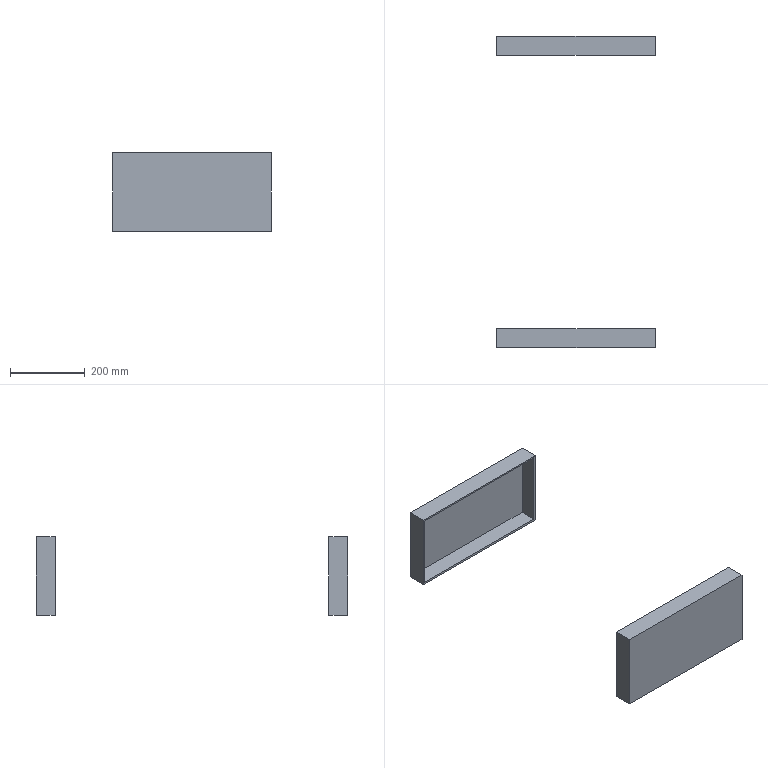Part | NX | features BREP 2 | 2 solids | 22 faces | box 422.751 x 830 x 210 mm | volume 1448252 mm3 | plane 22
STEP:
#1=CARTESIAN_POINT('',(-423.343,-172.553,205.));
#2=VERTEX_POINT('',#1);
#3=CARTESIAN_POINT('',(-423.343,-172.553,5.));
#4=VERTEX_POINT('',#3);
#5=CARTESIAN_POINT('',(-423.343,-172.553,210.));
#6=DIRECTION('',(0.,0.,-1.));
#7=VECTOR('',#6,1000.);
#8=LINE('',#5,#7);
#9=EDGE_CURVE('',#2,#4,#8,.T.);
#10=ORIENTED_EDGE('',*,*,#9,.F.);
#11=CARTESIAN_POINT('',(-423.343,-217.553,205.));
#12=VERTEX_POINT('',#11);
#13=CARTESIAN_POINT('',(-423.343,-167.553,205.));
#14=DIRECTION('',(0.,-1.,0.));
#15=VECTOR('',#14,1000.);
#16=LINE('',#13,#15);
#17=EDGE_CURVE('',#2,#12,#16,.T.);
#18=ORIENTED_EDGE('',*,*,#17,.T.);
#19=CARTESIAN_POINT('',(-423.343,-217.553,5.));
#20=VERTEX_POINT('',#19);
#21=CARTESIAN_POINT('',(-423.343,-217.553,210.));
#22=DIRECTION('',(0.,0.,1.));
#23=VECTOR('',#22,1000.);
#24=LINE('',#21,#23);
#25=EDGE_CURVE('',#20,#12,#24,.T.);
#26=ORIENTED_EDGE('',*,*,#25,.F.);
#27=CARTESIAN_POINT('',(-423.343,-167.553,5.));
#28=DIRECTION('',(0.,-1.,0.));
#29=VECTOR('',#28,1000.);
#30=LINE('',#27,#29);
#31=EDGE_CURVE('',#4,#20,#30,.T.);
#32=ORIENTED_EDGE('',*,*,#31,.F.);
#33=EDGE_LOOP('',(#10,#18,#26,#32));
#34=FACE_BOUND('',#33,.T.);
#35=CARTESIAN_POINT('',(-423.343,-167.553,210.));
#36=DIRECTION('',(1.,0.,0.));
#37=DIRECTION('',(0.,-1.,0.));
#38=AXIS2_PLACEMENT_3D('',#35,#36,#37);
#39=PLANE('',#38);
#40=ADVANCED_FACE('',(#34),#39,.T.);
#41=CARTESIAN_POINT('',(-10.592,-172.553,205.));
#42=VERTEX_POINT('',#41);
#43=CARTESIAN_POINT('',(-10.592,-172.553,5.));
#44=VERTEX_POINT('',#43);
#45=CARTESIAN_POINT('',(-10.592,-172.553,210.));
#46=DIRECTION('',(0.,0.,-1.));
#47=VECTOR('',#46,1000.);
#48=LINE('',#45,#47);
#49=EDGE_CURVE('',#42,#44,#48,.T.);
#50=ORIENTED_EDGE('',*,*,#49,.F.);
#51=CARTESIAN_POINT('',(-5.592,-172.553,205.));
#52=DIRECTION('',(-1.,0.,0.));
#53=VECTOR('',#52,1000.);
#54=LINE('',#51,#53);
#55=EDGE_CURVE('',#42,#2,#54,.T.);
#56=ORIENTED_EDGE('',*,*,#55,.T.);
#57=ORIENTED_EDGE('',*,*,#9,.T.);
#58=CARTESIAN_POINT('',(-5.592,-172.553,5.));
#59=DIRECTION('',(-1.,0.,0.));
#60=VECTOR('',#59,1000.);
#61=LINE('',#58,#60);
#62=EDGE_CURVE('',#44,#4,#61,.T.);
#63=ORIENTED_EDGE('',*,*,#62,.F.);
#64=EDGE_LOOP('',(#50,#56,#57,#63));
#65=FACE_BOUND('',#64,.T.);
#66=CARTESIAN_POINT('',(-5.592,-172.553,210.));
#67=DIRECTION('',(0.,-1.,0.));
#68=DIRECTION('',(-1.,0.,0.));
#69=AXIS2_PLACEMENT_3D('',#66,#67,#68);
#70=PLANE('',#69);
#71=ADVANCED_FACE('',(#65),#70,.T.);
#72=CARTESIAN_POINT('',(-10.592,-217.553,205.));
#73=VERTEX_POINT('',#72);
#74=CARTESIAN_POINT('',(-10.592,-217.553,5.));
#75=VERTEX_POINT('',#74);
#76=CARTESIAN_POINT('',(-10.592,-217.553,210.));
#77=DIRECTION('',(0.,0.,-1.));
#78=VECTOR('',#77,1000.);
#79=LINE('',#76,#78);
#80=EDGE_CURVE('',#73,#75,#79,.T.);
#81=ORIENTED_EDGE('',*,*,#80,.F.);
#82=CARTESIAN_POINT('',(-10.592,-217.553,205.));
#83=DIRECTION('',(0.,1.,0.));
#84=VECTOR('',#83,1000.);
#85=LINE('',#82,#84);
#86=EDGE_CURVE('',#73,#42,#85,.T.);
#87=ORIENTED_EDGE('',*,*,#86,.T.);
#88=ORIENTED_EDGE('',*,*,#49,.T.);
#89=CARTESIAN_POINT('',(-10.592,-217.553,5.));
#90=DIRECTION('',(0.,1.,0.));
#91=VECTOR('',#90,1000.);
#92=LINE('',#89,#91);
#93=EDGE_CURVE('',#75,#44,#92,.T.);
#94=ORIENTED_EDGE('',*,*,#93,.F.);
#95=EDGE_LOOP('',(#81,#87,#88,#94));
#96=FACE_BOUND('',#95,.T.);
#97=CARTESIAN_POINT('',(-10.592,-217.553,210.));
#98=DIRECTION('',(-1.,0.,0.));
#99=DIRECTION('',(0.,1.,0.));
#100=AXIS2_PLACEMENT_3D('',#97,#98,#99);
#101=PLANE('',#100);
#102=ADVANCED_FACE('',(#96),#101,.T.);
#103=CARTESIAN_POINT('',(-5.592,-217.553,210.));
#104=VERTEX_POINT('',#103);
#105=CARTESIAN_POINT('',(-428.343,-217.553,210.));
#106=VERTEX_POINT('',#105);
#107=CARTESIAN_POINT('',(-428.343,-217.553,210.));
#108=DIRECTION('',(-1.,0.,0.));
#109=VECTOR('',#108,1000.);
#110=LINE('',#107,#109);
#111=EDGE_CURVE('',#104,#106,#110,.T.);
#112=ORIENTED_EDGE('',*,*,#111,.F.);
#113=CARTESIAN_POINT('',(-5.592,-167.553,210.));
#114=VERTEX_POINT('',#113);
#115=CARTESIAN_POINT('',(-5.592,-217.553,210.));
#116=DIRECTION('',(0.,-1.,0.));
#117=VECTOR('',#116,1000.);
#118=LINE('',#115,#117);
#119=EDGE_CURVE('',#114,#104,#118,.T.);
#120=ORIENTED_EDGE('',*,*,#119,.F.);
#121=CARTESIAN_POINT('',(-428.343,-167.553,210.));
#122=VERTEX_POINT('',#121);
#123=CARTESIAN_POINT('',(-5.592,-167.553,210.));
#124=DIRECTION('',(1.,0.,0.));
#125=VECTOR('',#124,1000.);
#126=LINE('',#123,#125);
#127=EDGE_CURVE('',#122,#114,#126,.T.);
#128=ORIENTED_EDGE('',*,*,#127,.F.);
#129=CARTESIAN_POINT('',(-428.343,-167.553,210.));
#130=DIRECTION('',(0.,1.,0.));
#131=VECTOR('',#130,1000.);
#132=LINE('',#129,#131);
#133=EDGE_CURVE('',#106,#122,#132,.T.);
#134=ORIENTED_EDGE('',*,*,#133,.F.);
#135=EDGE_LOOP('',(#112,#120,#128,#134));
#136=FACE_BOUND('',#135,.T.);
#137=CARTESIAN_POINT('',(-428.343,-167.553,210.));
#138=DIRECTION('',(0.,0.,1.));
#139=DIRECTION('',(0.,1.,0.));
#140=AXIS2_PLACEMENT_3D('',#137,#138,#139);
#141=PLANE('',#140);
#142=ADVANCED_FACE('',(#136),#141,.T.);
#143=CARTESIAN_POINT('',(-5.592,-217.553,0.));
#144=VERTEX_POINT('',#143);
#145=CARTESIAN_POINT('',(-428.343,-217.553,0.));
#146=VERTEX_POINT('',#145);
#147=CARTESIAN_POINT('',(-428.343,-217.553,0.));
#148=DIRECTION('',(-1.,0.,0.));
#149=VECTOR('',#148,1000.);
#150=LINE('',#147,#149);
#151=EDGE_CURVE('',#144,#146,#150,.T.);
#152=ORIENTED_EDGE('',*,*,#151,.F.);
#153=CARTESIAN_POINT('',(-5.592,-217.553,210.));
#154=DIRECTION('',(0.,0.,-1.));
#155=VECTOR('',#154,1000.);
#156=LINE('',#153,#155);
#157=EDGE_CURVE('',#104,#144,#156,.T.);
#158=ORIENTED_EDGE('',*,*,#157,.F.);
#159=ORIENTED_EDGE('',*,*,#111,.T.);
#160=CARTESIAN_POINT('',(-428.343,-217.553,210.));
#161=DIRECTION('',(0.,0.,1.));
#162=VECTOR('',#161,1000.);
#163=LINE('',#160,#162);
#164=EDGE_CURVE('',#146,#106,#163,.T.);
#165=ORIENTED_EDGE('',*,*,#164,.F.);
#166=EDGE_LOOP('',(#152,#158,#159,#165));
#167=FACE_BOUND('',#166,.T.);
#168=ORIENTED_EDGE('',*,*,#80,.T.);
#169=CARTESIAN_POINT('',(-428.343,-217.553,5.));
#170=DIRECTION('',(1.,0.,0.));
#171=VECTOR('',#170,1000.);
#172=LINE('',#169,#171);
#173=EDGE_CURVE('',#20,#75,#172,.T.);
#174=ORIENTED_EDGE('',*,*,#173,.F.);
#175=ORIENTED_EDGE('',*,*,#25,.T.);
#176=CARTESIAN_POINT('',(-37.592,-217.553,205.));
#177=DIRECTION('',(1.,0.,0.));
#178=VECTOR('',#177,1000.);
#179=LINE('',#176,#178);
#180=EDGE_CURVE('',#12,#73,#179,.T.);
#181=ORIENTED_EDGE('',*,*,#180,.T.);
#182=EDGE_LOOP('',(#168,#174,#175,#181));
#183=FACE_BOUND('',#182,.T.);
#184=CARTESIAN_POINT('',(-428.343,-217.553,210.));
#185=DIRECTION('',(0.,-1.,0.));
#186=DIRECTION('',(0.,0.,1.));
#187=AXIS2_PLACEMENT_3D('',#184,#185,#186);
#188=PLANE('',#187);
#189=ADVANCED_FACE('',(#167,#183),#188,.T.);
#190=CARTESIAN_POINT('',(-5.592,-167.553,0.));
#191=VERTEX_POINT('',#190);
#192=CARTESIAN_POINT('',(-5.592,-217.553,0.));
#193=DIRECTION('',(0.,1.,0.));
#194=VECTOR('',#193,1000.);
#195=LINE('',#192,#194);
#196=EDGE_CURVE('',#144,#191,#195,.T.);
#197=ORIENTED_EDGE('',*,*,#196,.F.);
#198=ORIENTED_EDGE('',*,*,#151,.T.);
#199=CARTESIAN_POINT('',(-428.343,-167.553,0.));
#200=VERTEX_POINT('',#199);
#201=CARTESIAN_POINT('',(-428.343,-167.553,0.));
#202=DIRECTION('',(0.,-1.,0.));
#203=VECTOR('',#202,1000.);
#204=LINE('',#201,#203);
#205=EDGE_CURVE('',#200,#146,#204,.T.);
#206=ORIENTED_EDGE('',*,*,#205,.F.);
#207=CARTESIAN_POINT('',(-5.592,-167.553,0.));
#208=DIRECTION('',(-1.,0.,0.));
#209=VECTOR('',#208,1000.);
#210=LINE('',#207,#209);
#211=EDGE_CURVE('',#191,#200,#210,.T.);
#212=ORIENTED_EDGE('',*,*,#211,.F.);
#213=EDGE_LOOP('',(#197,#198,#206,#212));
#214=FACE_BOUND('',#213,.T.);
#215=CARTESIAN_POINT('',(-5.592,-167.553,0.));
#216=DIRECTION('',(0.,0.,1.));
#217=DIRECTION('',(1.,0.,0.));
#218=AXIS2_PLACEMENT_3D('',#215,#216,#217);
#219=PLANE('',#218);
#220=ADVANCED_FACE('',(#214),#219,.F.);
#221=CARTESIAN_POINT('',(-428.343,-167.553,210.));
#222=DIRECTION('',(0.,0.,-1.));
#223=VECTOR('',#222,1000.);
#224=LINE('',#221,#223);
#225=EDGE_CURVE('',#122,#200,#224,.T.);
#226=ORIENTED_EDGE('',*,*,#225,.T.);
#227=ORIENTED_EDGE('',*,*,#205,.T.);
#228=ORIENTED_EDGE('',*,*,#164,.T.);
#229=ORIENTED_EDGE('',*,*,#133,.T.);
#230=EDGE_LOOP('',(#226,#227,#228,#229));
#231=FACE_BOUND('',#230,.T.);
#232=CARTESIAN_POINT('',(-428.343,-167.553,210.));
#233=DIRECTION('',(1.,0.,0.));
#234=DIRECTION('',(0.,-1.,0.));
#235=AXIS2_PLACEMENT_3D('',#232,#233,#234);
#236=PLANE('',#235);
#237=ADVANCED_FACE('',(#231),#236,.F.);
#238=CARTESIAN_POINT('',(-5.592,-167.553,210.));
#239=DIRECTION('',(0.,0.,-1.));
#240=VECTOR('',#239,1000.);
#241=LINE('',#238,#240);
#242=EDGE_CURVE('',#114,#191,#241,.T.);
#243=ORIENTED_EDGE('',*,*,#242,.T.);
#244=ORIENTED_EDGE('',*,*,#211,.T.);
#245=ORIENTED_EDGE('',*,*,#225,.F.);
#246=ORIENTED_EDGE('',*,*,#127,.T.);
#247=EDGE_LOOP('',(#243,#244,#245,#246));
#248=FACE_BOUND('',#247,.T.);
#249=CARTESIAN_POINT('',(-5.592,-167.553,210.));
#250=DIRECTION('',(0.,-1.,0.));
#251=DIRECTION('',(-1.,0.,0.));
#252=AXIS2_PLACEMENT_3D('',#249,#250,#251);
#253=PLANE('',#252);
#254=ADVANCED_FACE('',(#248),#253,.F.);
#255=ORIENTED_EDGE('',*,*,#157,.T.);
#256=ORIENTED_EDGE('',*,*,#196,.T.);
#257=ORIENTED_EDGE('',*,*,#242,.F.);
#258=ORIENTED_EDGE('',*,*,#119,.T.);
#259=EDGE_LOOP('',(#255,#256,#257,#258));
#260=FACE_BOUND('',#259,.T.);
#261=CARTESIAN_POINT('',(-5.592,-217.553,210.));
#262=DIRECTION('',(-1.,0.,0.));
#263=DIRECTION('',(0.,1.,0.));
#264=AXIS2_PLACEMENT_3D('',#261,#262,#263);
#265=PLANE('',#264);
#266=ADVANCED_FACE('',(#260),#265,.F.);
#267=ORIENTED_EDGE('',*,*,#62,.T.);
#268=ORIENTED_EDGE('',*,*,#31,.T.);
#269=ORIENTED_EDGE('',*,*,#173,.T.);
#270=ORIENTED_EDGE('',*,*,#93,.T.);
#271=EDGE_LOOP('',(#267,#268,#269,#270));
#272=FACE_BOUND('',#271,.T.);
#273=CARTESIAN_POINT('',(0.,0.,5.));
#274=DIRECTION('',(0.,0.,1.));
#275=DIRECTION('',(-1.,0.,0.));
#276=AXIS2_PLACEMENT_3D('',#273,#274,#275);
#277=PLANE('',#276);
#278=ADVANCED_FACE('',(#272),#277,.T.);
#279=ORIENTED_EDGE('',*,*,#17,.F.);
#280=ORIENTED_EDGE('',*,*,#55,.F.);
#281=ORIENTED_EDGE('',*,*,#86,.F.);
#282=ORIENTED_EDGE('',*,*,#180,.F.);
#283=EDGE_LOOP('',(#279,#280,#281,#282));
#284=FACE_BOUND('',#283,.T.);
#285=CARTESIAN_POINT('',(0.,0.,205.));
#286=DIRECTION('',(0.,0.,1.));
#287=DIRECTION('',(-1.,0.,0.));
#288=AXIS2_PLACEMENT_3D('',#285,#286,#287);
#289=PLANE('',#288);
#290=ADVANCED_FACE('',(#284),#289,.F.);
#291=CLOSED_SHELL('',(#40,#71,#102,#142,#189,#220,#237,#254,#266,#278,#290));
#292=MANIFOLD_SOLID_BREP('',#291);
#293=CARTESIAN_POINT('',(-423.343,-992.553,205.));
#294=VERTEX_POINT('',#293);
#295=CARTESIAN_POINT('',(-423.343,-947.553,205.));
#296=VERTEX_POINT('',#295);
#297=CARTESIAN_POINT('',(-423.343,-997.553,205.));
#298=DIRECTION('',(0.,1.,0.));
#299=VECTOR('',#298,1000.);
#300=LINE('',#297,#299);
#301=EDGE_CURVE('',#294,#296,#300,.T.);
#302=ORIENTED_EDGE('',*,*,#301,.F.);
#303=CARTESIAN_POINT('',(-423.343,-992.553,5.));
#304=VERTEX_POINT('',#303);
#305=CARTESIAN_POINT('',(-423.343,-992.553,210.));
#306=DIRECTION('',(0.,0.,-1.));
#307=VECTOR('',#306,1000.);
#308=LINE('',#305,#307);
#309=EDGE_CURVE('',#294,#304,#308,.T.);
#310=ORIENTED_EDGE('',*,*,#309,.T.);
#311=CARTESIAN_POINT('',(-423.343,-947.553,5.));
#312=VERTEX_POINT('',#311);
#313=CARTESIAN_POINT('',(-423.343,-997.553,5.));
#314=DIRECTION('',(0.,-1.,0.));
#315=VECTOR('',#314,1000.);
#316=LINE('',#313,#315);
#317=EDGE_CURVE('',#312,#304,#316,.T.);
#318=ORIENTED_EDGE('',*,*,#317,.F.);
#319=CARTESIAN_POINT('',(-423.343,-947.553,210.));
#320=DIRECTION('',(0.,0.,1.));
#321=VECTOR('',#320,1000.);
#322=LINE('',#319,#321);
#323=EDGE_CURVE('',#312,#296,#322,.T.);
#324=ORIENTED_EDGE('',*,*,#323,.T.);
#325=EDGE_LOOP('',(#302,#310,#318,#324));
#326=FACE_BOUND('',#325,.T.);
#327=CARTESIAN_POINT('',(-423.343,-997.553,210.));
#328=DIRECTION('',(-1.,0.,0.));
#329=DIRECTION('',(0.,1.,0.));
#330=AXIS2_PLACEMENT_3D('',#327,#328,#329);
#331=PLANE('',#330);
#332=ADVANCED_FACE('',(#326),#331,.F.);
#333=CARTESIAN_POINT('',(-10.592,-992.553,205.));
#334=VERTEX_POINT('',#333);
#335=CARTESIAN_POINT('',(-5.592,-992.553,205.));
#336=DIRECTION('',(-1.,0.,0.));
#337=VECTOR('',#336,1000.);
#338=LINE('',#335,#337);
#339=EDGE_CURVE('',#334,#294,#338,.T.);
#340=ORIENTED_EDGE('',*,*,#339,.F.);
#341=CARTESIAN_POINT('',(-10.592,-992.553,5.));
#342=VERTEX_POINT('',#341);
#343=CARTESIAN_POINT('',(-10.592,-992.553,210.));
#344=DIRECTION('',(0.,0.,-1.));
#345=VECTOR('',#344,1000.);
#346=LINE('',#343,#345);
#347=EDGE_CURVE('',#334,#342,#346,.T.);
#348=ORIENTED_EDGE('',*,*,#347,.T.);
#349=CARTESIAN_POINT('',(-5.592,-992.553,5.));
#350=DIRECTION('',(1.,0.,0.));
#351=VECTOR('',#350,1000.);
#352=LINE('',#349,#351);
#353=EDGE_CURVE('',#304,#342,#352,.T.);
#354=ORIENTED_EDGE('',*,*,#353,.F.);
#355=ORIENTED_EDGE('',*,*,#309,.F.);
#356=EDGE_LOOP('',(#340,#348,#354,#355));
#357=FACE_BOUND('',#356,.T.);
#358=CARTESIAN_POINT('',(-5.592,-992.553,210.));
#359=DIRECTION('',(0.,-1.,0.));
#360=DIRECTION('',(-1.,0.,0.));
#361=AXIS2_PLACEMENT_3D('',#358,#359,#360);
#362=PLANE('',#361);
#363=ADVANCED_FACE('',(#357),#362,.F.);
#364=CARTESIAN_POINT('',(-10.592,-947.553,205.));
#365=VERTEX_POINT('',#364);
#366=CARTESIAN_POINT('',(-10.592,-947.553,205.));
#367=DIRECTION('',(0.,-1.,0.));
#368=VECTOR('',#367,1000.);
#369=LINE('',#366,#368);
#370=EDGE_CURVE('',#365,#334,#369,.T.);
#371=ORIENTED_EDGE('',*,*,#370,.F.);
#372=CARTESIAN_POINT('',(-10.592,-947.553,5.));
#373=VERTEX_POINT('',#372);
#374=CARTESIAN_POINT('',(-10.592,-947.553,210.));
#375=DIRECTION('',(0.,0.,-1.));
#376=VECTOR('',#375,1000.);
#377=LINE('',#374,#376);
#378=EDGE_CURVE('',#365,#373,#377,.T.);
#379=ORIENTED_EDGE('',*,*,#378,.T.);
#380=CARTESIAN_POINT('',(-10.592,-947.553,5.));
#381=DIRECTION('',(0.,1.,0.));
#382=VECTOR('',#381,1000.);
#383=LINE('',#380,#382);
#384=EDGE_CURVE('',#342,#373,#383,.T.);
#385=ORIENTED_EDGE('',*,*,#384,.F.);
#386=ORIENTED_EDGE('',*,*,#347,.F.);
#387=EDGE_LOOP('',(#371,#379,#385,#386));
#388=FACE_BOUND('',#387,.T.);
#389=CARTESIAN_POINT('',(-10.592,-947.553,210.));
#390=DIRECTION('',(1.,0.,0.));
#391=DIRECTION('',(0.,-1.,0.));
#392=AXIS2_PLACEMENT_3D('',#389,#390,#391);
#393=PLANE('',#392);
#394=ADVANCED_FACE('',(#388),#393,.F.);
#395=CARTESIAN_POINT('',(-428.343,-947.553,210.));
#396=VERTEX_POINT('',#395);
#397=CARTESIAN_POINT('',(-5.592,-947.553,210.));
#398=VERTEX_POINT('',#397);
#399=CARTESIAN_POINT('',(-5.592,-947.553,210.));
#400=DIRECTION('',(1.,0.,0.));
#401=VECTOR('',#400,1000.);
#402=LINE('',#399,#401);
#403=EDGE_CURVE('',#396,#398,#402,.T.);
#404=ORIENTED_EDGE('',*,*,#403,.F.);
#405=CARTESIAN_POINT('',(-428.343,-997.553,210.));
#406=VERTEX_POINT('',#405);
#407=CARTESIAN_POINT('',(-428.343,-997.553,210.));
#408=DIRECTION('',(0.,-1.,0.));
#409=VECTOR('',#408,1000.);
#410=LINE('',#407,#409);
#411=EDGE_CURVE('',#396,#406,#410,.T.);
#412=ORIENTED_EDGE('',*,*,#411,.T.);
#413=CARTESIAN_POINT('',(-5.592,-997.553,210.));
#414=VERTEX_POINT('',#413);
#415=CARTESIAN_POINT('',(-5.592,-997.553,210.));
#416=DIRECTION('',(1.,0.,0.));
#417=VECTOR('',#416,1000.);
#418=LINE('',#415,#417);
#419=EDGE_CURVE('',#406,#414,#418,.T.);
#420=ORIENTED_EDGE('',*,*,#419,.T.);
#421=CARTESIAN_POINT('',(-5.592,-947.553,210.));
#422=DIRECTION('',(0.,1.,0.));
#423=VECTOR('',#422,1000.);
#424=LINE('',#421,#423);
#425=EDGE_CURVE('',#414,#398,#424,.T.);
#426=ORIENTED_EDGE('',*,*,#425,.T.);
#427=EDGE_LOOP('',(#404,#412,#420,#426));
#428=FACE_BOUND('',#427,.T.);
#429=CARTESIAN_POINT('',(-5.592,-947.553,210.));
#430=DIRECTION('',(0.,0.,1.));
#431=DIRECTION('',(0.,1.,0.));
#432=AXIS2_PLACEMENT_3D('',#429,#430,#431);
#433=PLANE('',#432);
#434=ADVANCED_FACE('',(#428),#433,.T.);
#435=CARTESIAN_POINT('',(-428.343,-947.553,0.));
#436=VERTEX_POINT('',#435);
#437=CARTESIAN_POINT('',(-5.592,-947.553,0.));
#438=VERTEX_POINT('',#437);
#439=CARTESIAN_POINT('',(-428.343,-947.553,0.));
#440=DIRECTION('',(1.,0.,0.));
#441=VECTOR('',#440,1000.);
#442=LINE('',#439,#441);
#443=EDGE_CURVE('',#436,#438,#442,.T.);
#444=ORIENTED_EDGE('',*,*,#443,.T.);
#445=CARTESIAN_POINT('',(-5.592,-997.553,0.));
#446=VERTEX_POINT('',#445);
#447=CARTESIAN_POINT('',(-5.592,-947.553,0.));
#448=DIRECTION('',(0.,-1.,0.));
#449=VECTOR('',#448,1000.);
#450=LINE('',#447,#449);
#451=EDGE_CURVE('',#438,#446,#450,.T.);
#452=ORIENTED_EDGE('',*,*,#451,.T.);
#453=CARTESIAN_POINT('',(-428.343,-997.553,0.));
#454=VERTEX_POINT('',#453);
#455=CARTESIAN_POINT('',(-5.592,-997.553,0.));
#456=DIRECTION('',(-1.,0.,0.));
#457=VECTOR('',#456,1000.);
#458=LINE('',#455,#457);
#459=EDGE_CURVE('',#446,#454,#458,.T.);
#460=ORIENTED_EDGE('',*,*,#459,.T.);
#461=CARTESIAN_POINT('',(-428.343,-997.553,0.));
#462=DIRECTION('',(0.,1.,0.));
#463=VECTOR('',#462,1000.);
#464=LINE('',#461,#463);
#465=EDGE_CURVE('',#454,#436,#464,.T.);
#466=ORIENTED_EDGE('',*,*,#465,.T.);
#467=EDGE_LOOP('',(#444,#452,#460,#466));
#468=FACE_BOUND('',#467,.T.);
#469=CARTESIAN_POINT('',(-428.343,-997.553,0.));
#470=DIRECTION('',(0.,0.,1.));
#471=DIRECTION('',(0.,-1.,0.));
#472=AXIS2_PLACEMENT_3D('',#469,#470,#471);
#473=PLANE('',#472);
#474=ADVANCED_FACE('',(#468),#473,.F.);
#475=CARTESIAN_POINT('',(-5.592,-947.553,210.));
#476=DIRECTION('',(0.,0.,-1.));
#477=VECTOR('',#476,1000.);
#478=LINE('',#475,#477);
#479=EDGE_CURVE('',#398,#438,#478,.T.);
#480=ORIENTED_EDGE('',*,*,#479,.T.);
#481=ORIENTED_EDGE('',*,*,#443,.F.);
#482=CARTESIAN_POINT('',(-428.343,-947.553,210.));
#483=DIRECTION('',(0.,0.,1.));
#484=VECTOR('',#483,1000.);
#485=LINE('',#482,#484);
#486=EDGE_CURVE('',#436,#396,#485,.T.);
#487=ORIENTED_EDGE('',*,*,#486,.T.);
#488=ORIENTED_EDGE('',*,*,#403,.T.);
#489=EDGE_LOOP('',(#480,#481,#487,#488));
#490=FACE_BOUND('',#489,.T.);
#491=CARTESIAN_POINT('',(-396.343,-947.553,5.));
#492=DIRECTION('',(-1.,0.,0.));
#493=VECTOR('',#492,1000.);
#494=LINE('',#491,#493);
#495=EDGE_CURVE('',#373,#312,#494,.T.);
#496=ORIENTED_EDGE('',*,*,#495,.F.);
#497=ORIENTED_EDGE('',*,*,#378,.F.);
#498=CARTESIAN_POINT('',(-5.592,-947.553,205.));
#499=DIRECTION('',(-1.,0.,0.));
#500=VECTOR('',#499,1000.);
#501=LINE('',#498,#500);
#502=EDGE_CURVE('',#365,#296,#501,.T.);
#503=ORIENTED_EDGE('',*,*,#502,.T.);
#504=ORIENTED_EDGE('',*,*,#323,.F.);
#505=EDGE_LOOP('',(#496,#497,#503,#504));
#506=FACE_BOUND('',#505,.T.);
#507=CARTESIAN_POINT('',(-428.343,-947.553,210.));
#508=DIRECTION('',(0.,1.,0.));
#509=DIRECTION('',(0.,0.,1.));
#510=AXIS2_PLACEMENT_3D('',#507,#508,#509);
#511=PLANE('',#510);
#512=ADVANCED_FACE('',(#490,#506),#511,.T.);
#513=ORIENTED_EDGE('',*,*,#465,.F.);
#514=CARTESIAN_POINT('',(-428.343,-997.553,210.));
#515=DIRECTION('',(0.,0.,-1.));
#516=VECTOR('',#515,1000.);
#517=LINE('',#514,#516);
#518=EDGE_CURVE('',#406,#454,#517,.T.);
#519=ORIENTED_EDGE('',*,*,#518,.F.);
#520=ORIENTED_EDGE('',*,*,#411,.F.);
#521=ORIENTED_EDGE('',*,*,#486,.F.);
#522=EDGE_LOOP('',(#513,#519,#520,#521));
#523=FACE_BOUND('',#522,.T.);
#524=CARTESIAN_POINT('',(-428.343,-997.553,210.));
#525=DIRECTION('',(-1.,0.,0.));
#526=DIRECTION('',(0.,1.,0.));
#527=AXIS2_PLACEMENT_3D('',#524,#525,#526);
#528=PLANE('',#527);
#529=ADVANCED_FACE('',(#523),#528,.T.);
#530=ORIENTED_EDGE('',*,*,#459,.F.);
#531=CARTESIAN_POINT('',(-5.592,-997.553,210.));
#532=DIRECTION('',(0.,0.,-1.));
#533=VECTOR('',#532,1000.);
#534=LINE('',#531,#533);
#535=EDGE_CURVE('',#414,#446,#534,.T.);
#536=ORIENTED_EDGE('',*,*,#535,.F.);
#537=ORIENTED_EDGE('',*,*,#419,.F.);
#538=ORIENTED_EDGE('',*,*,#518,.T.);
#539=EDGE_LOOP('',(#530,#536,#537,#538));
#540=FACE_BOUND('',#539,.T.);
#541=CARTESIAN_POINT('',(-5.592,-997.553,210.));
#542=DIRECTION('',(0.,-1.,0.));
#543=DIRECTION('',(-1.,0.,0.));
#544=AXIS2_PLACEMENT_3D('',#541,#542,#543);
#545=PLANE('',#544);
#546=ADVANCED_FACE('',(#540),#545,.T.);
#547=ORIENTED_EDGE('',*,*,#451,.F.);
#548=ORIENTED_EDGE('',*,*,#479,.F.);
#549=ORIENTED_EDGE('',*,*,#425,.F.);
#550=ORIENTED_EDGE('',*,*,#535,.T.);
#551=EDGE_LOOP('',(#547,#548,#549,#550));
#552=FACE_BOUND('',#551,.T.);
#553=CARTESIAN_POINT('',(-5.592,-947.553,210.));
#554=DIRECTION('',(1.,0.,0.));
#555=DIRECTION('',(0.,-1.,0.));
#556=AXIS2_PLACEMENT_3D('',#553,#554,#555);
#557=PLANE('',#556);
#558=ADVANCED_FACE('',(#552),#557,.T.);
#559=ORIENTED_EDGE('',*,*,#495,.T.);
#560=ORIENTED_EDGE('',*,*,#317,.T.);
#561=ORIENTED_EDGE('',*,*,#353,.T.);
#562=ORIENTED_EDGE('',*,*,#384,.T.);
#563=EDGE_LOOP('',(#559,#560,#561,#562));
#564=FACE_BOUND('',#563,.T.);
#565=CARTESIAN_POINT('',(0.,0.,5.));
#566=DIRECTION('',(0.,0.,-1.));
#567=DIRECTION('',(1.,0.,0.));
#568=AXIS2_PLACEMENT_3D('',#565,#566,#567);
#569=PLANE('',#568);
#570=ADVANCED_FACE('',(#564),#569,.F.);
#571=ORIENTED_EDGE('',*,*,#339,.T.);
#572=ORIENTED_EDGE('',*,*,#301,.T.);
#573=ORIENTED_EDGE('',*,*,#502,.F.);
#574=ORIENTED_EDGE('',*,*,#370,.T.);
#575=EDGE_LOOP('',(#571,#572,#573,#574));
#576=FACE_BOUND('',#575,.T.);
#577=CARTESIAN_POINT('',(0.,0.,205.));
#578=DIRECTION('',(0.,0.,1.));
#579=DIRECTION('',(-1.,0.,0.));
#580=AXIS2_PLACEMENT_3D('',#577,#578,#579);
#581=PLANE('',#580);
#582=ADVANCED_FACE('',(#576),#581,.F.);
#583=CLOSED_SHELL('',(#332,#363,#394,#434,#474,#512,#529,#546,#558,#570,#582));
#584=MANIFOLD_SOLID_BREP('',#583);
#585=(LENGTH_UNIT()NAMED_UNIT(*)SI_UNIT(.MILLI.,.METRE.));
#586=UNCERTAINTY_MEASURE_WITH_UNIT(LENGTH_MEASURE(0.00001),#585,'','');
#587=(NAMED_UNIT(*)PLANE_ANGLE_UNIT()SI_UNIT($,.RADIAN.));
#588=(NAMED_UNIT(*)SI_UNIT($,.STERADIAN.)SOLID_ANGLE_UNIT());
#589=(GEOMETRIC_REPRESENTATION_CONTEXT(3)GLOBAL_UNCERTAINTY_ASSIGNED_CONTEXT((#586))GLOBAL_UNIT_ASSIGNED_CONTEXT((#585,#587,#588))REPRESENTATION_CONTEXT('',''));
#590=ADVANCED_BREP_SHAPE_REPRESENTATION('',(#292,#584),#589);